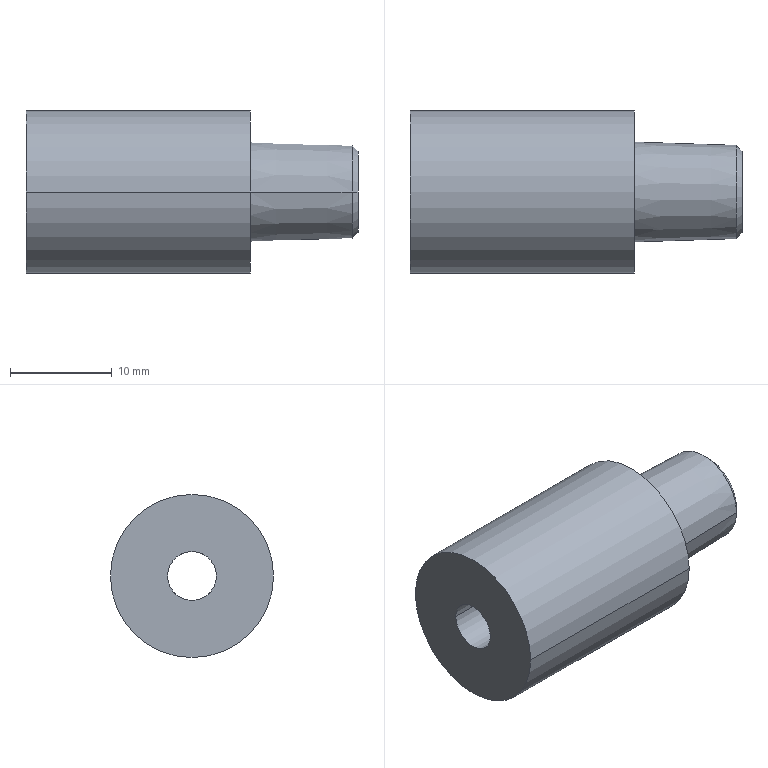Part | Creo | 1 solid | 21 faces | box 32.58 x 16 x 16 mm | volume 4565 mm3 | plane 11 | cylinder 6 | cone 4 | commonest cylinder face diameters 4.8 x4 16 x2
STEP:
#1=CARTESIAN_POINT('',(-305.,-184.66,90.));
#2=VERTEX_POINT('',#1);
#3=CARTESIAN_POINT('',(-305.,-175.5,90.));
#4=VERTEX_POINT('',#3);
#5=CARTESIAN_POINT('',(-305.,-180.08,90.));
#6=DIRECTION('',(-1.,0.,0.));
#7=DIRECTION('',(0.,-1.,0.));
#8=AXIS2_PLACEMENT_3D('',#5,#6,#7);
#9=CIRCLE('',#8,4.58);
#10=EDGE_CURVE('',#2,#4,#9,.T.);
#11=ORIENTED_EDGE('',*,*,#10,.F.);
#12=CARTESIAN_POINT('',(-315.,-184.98,90.));
#13=VERTEX_POINT('',#12);
#14=CARTESIAN_POINT('',(-305.,-184.66,90.));
#15=DIRECTION('',(-0.9995,-0.03198,0.));
#16=VECTOR('',#15,10.005);
#17=LINE('',#14,#16);
#18=EDGE_CURVE('',#2,#13,#17,.T.);
#19=ORIENTED_EDGE('',*,*,#18,.T.);
#20=CARTESIAN_POINT('',(-315.,-175.18,90.));
#21=VERTEX_POINT('',#20);
#22=CARTESIAN_POINT('',(-315.,-180.08,90.));
#23=DIRECTION('',(-1.,0.,0.));
#24=DIRECTION('',(0.,-1.,0.));
#25=AXIS2_PLACEMENT_3D('',#22,#23,#24);
#26=CIRCLE('',#25,4.9);
#27=EDGE_CURVE('',#13,#21,#26,.T.);
#28=ORIENTED_EDGE('',*,*,#27,.T.);
#29=CARTESIAN_POINT('',(-305.,-175.5,90.));
#30=DIRECTION('',(-0.9995,0.03198,0.));
#31=VECTOR('',#30,10.005);
#32=LINE('',#29,#31);
#33=EDGE_CURVE('',#4,#21,#32,.T.);
#34=ORIENTED_EDGE('',*,*,#33,.F.);
#35=EDGE_LOOP('',(#11,#19,#28,#34));
#36=FACE_OUTER_BOUND('',#35,.F.);
#37=CARTESIAN_POINT('',(-310.,-180.08,90.));
#38=DIRECTION('',(-1.,0.,0.));
#39=DIRECTION('',(0.,-1.,0.));
#40=AXIS2_PLACEMENT_3D('',#37,#38,#39);
#41=CONICAL_SURFACE('',#40,4.74,1.833);
#42=ADVANCED_FACE('',(#36),#41,.T.);
#43=CARTESIAN_POINT('',(-304.42,-176.08,90.));
#44=VERTEX_POINT('',#43);
#45=CARTESIAN_POINT('',(-304.42,-184.08,90.));
#46=VERTEX_POINT('',#45);
#47=CARTESIAN_POINT('',(-304.42,-180.08,90.));
#48=DIRECTION('',(1.,0.,0.));
#49=DIRECTION('',(0.,1.,0.));
#50=AXIS2_PLACEMENT_3D('',#47,#48,#49);
#51=CIRCLE('',#50,4.);
#52=EDGE_CURVE('',#44,#46,#51,.T.);
#53=ORIENTED_EDGE('',*,*,#52,.T.);
#54=CARTESIAN_POINT('',(-304.42,-184.08,90.));
#55=DIRECTION('',(-0.7071,-0.7071,0.));
#56=VECTOR('',#55,0.8202);
#57=LINE('',#54,#56);
#58=EDGE_CURVE('',#46,#2,#57,.T.);
#59=ORIENTED_EDGE('',*,*,#58,.T.);
#60=ORIENTED_EDGE('',*,*,#10,.T.);
#61=CARTESIAN_POINT('',(-304.42,-176.08,90.));
#62=DIRECTION('',(-0.7071,0.7071,0.));
#63=VECTOR('',#62,0.8202);
#64=LINE('',#61,#63);
#65=EDGE_CURVE('',#44,#4,#64,.T.);
#66=ORIENTED_EDGE('',*,*,#65,.F.);
#67=EDGE_LOOP('',(#53,#59,#60,#66));
#68=FACE_OUTER_BOUND('',#67,.F.);
#69=CARTESIAN_POINT('',(-304.71,-180.08,90.));
#70=DIRECTION('',(-1.,0.,0.));
#71=DIRECTION('',(0.,-1.,0.));
#72=AXIS2_PLACEMENT_3D('',#69,#70,#71);
#73=CONICAL_SURFACE('',#72,4.29,45.);
#74=ADVANCED_FACE('',(#68),#73,.T.);
#75=CARTESIAN_POINT('',(-304.42,-180.08,90.));
#76=DIRECTION('',(1.,0.,0.));
#77=DIRECTION('',(0.,-1.,0.));
#78=AXIS2_PLACEMENT_3D('',#75,#76,#77);
#79=CIRCLE('',#78,4.);
#80=EDGE_CURVE('',#46,#44,#79,.T.);
#81=ORIENTED_EDGE('',*,*,#80,.F.);
#82=ORIENTED_EDGE('',*,*,#52,.F.);
#83=EDGE_LOOP('',(#81,#82));
#84=FACE_OUTER_BOUND('',#83,.F.);
#85=CARTESIAN_POINT('',(-304.42,-180.08,87.6));
#86=VERTEX_POINT('',#85);
#87=CARTESIAN_POINT('',(-304.42,-182.48,90.));
#88=VERTEX_POINT('',#87);
#89=CARTESIAN_POINT('',(-304.42,-180.08,90.));
#90=DIRECTION('',(-1.,0.,0.));
#91=DIRECTION('',(0.,0.,-1.));
#92=AXIS2_PLACEMENT_3D('',#89,#90,#91);
#93=CIRCLE('',#92,2.4);
#94=EDGE_CURVE('',#86,#88,#93,.T.);
#95=ORIENTED_EDGE('',*,*,#94,.F.);
#96=CARTESIAN_POINT('',(-304.42,-177.68,90.));
#97=VERTEX_POINT('',#96);
#98=CARTESIAN_POINT('',(-304.42,-180.08,90.));
#99=DIRECTION('',(-1.,0.,0.));
#100=DIRECTION('',(0.,1.,0.));
#101=AXIS2_PLACEMENT_3D('',#98,#99,#100);
#102=CIRCLE('',#101,2.4);
#103=EDGE_CURVE('',#97,#86,#102,.T.);
#104=ORIENTED_EDGE('',*,*,#103,.F.);
#105=CARTESIAN_POINT('',(-304.42,-180.08,90.));
#106=DIRECTION('',(-1.,0.,0.));
#107=DIRECTION('',(0.,-1.,0.));
#108=AXIS2_PLACEMENT_3D('',#105,#106,#107);
#109=CIRCLE('',#108,2.4);
#110=EDGE_CURVE('',#88,#97,#109,.T.);
#111=ORIENTED_EDGE('',*,*,#110,.F.);
#112=EDGE_LOOP('',(#95,#104,#111));
#113=FACE_BOUND('',#112,.F.);
#114=CARTESIAN_POINT('',(-304.42,-180.08,90.));
#115=DIRECTION('',(1.,0.,0.));
#116=DIRECTION('',(0.,0.,-1.));
#117=AXIS2_PLACEMENT_3D('',#114,#115,#116);
#118=PLANE('',#117);
#119=ADVANCED_FACE('',(#84,#113),#118,.T.);
#120=ORIENTED_EDGE('',*,*,#103,.T.);
#121=ORIENTED_EDGE('',*,*,#94,.T.);
#122=CARTESIAN_POINT('',(-312.,-182.48,90.));
#123=VERTEX_POINT('',#122);
#124=CARTESIAN_POINT('',(-312.,-182.48,90.));
#125=DIRECTION('',(1.,0.,0.));
#126=VECTOR('',#125,7.58);
#127=LINE('',#124,#126);
#128=EDGE_CURVE('',#123,#88,#127,.T.);
#129=ORIENTED_EDGE('',*,*,#128,.F.);
#130=CARTESIAN_POINT('',(-312.,-180.08,87.6));
#131=VERTEX_POINT('',#130);
#132=CARTESIAN_POINT('',(-312.,-180.08,90.));
#133=DIRECTION('',(1.,0.,0.));
#134=DIRECTION('',(0.,-1.,0.));
#135=AXIS2_PLACEMENT_3D('',#132,#133,#134);
#136=CIRCLE('',#135,2.4);
#137=EDGE_CURVE('',#123,#131,#136,.T.);
#138=ORIENTED_EDGE('',*,*,#137,.T.);
#139=CARTESIAN_POINT('',(-312.,-177.68,90.));
#140=VERTEX_POINT('',#139);
#141=CARTESIAN_POINT('',(-312.,-180.08,90.));
#142=DIRECTION('',(1.,0.,0.));
#143=DIRECTION('',(0.,0.,-1.));
#144=AXIS2_PLACEMENT_3D('',#141,#142,#143);
#145=CIRCLE('',#144,2.4);
#146=EDGE_CURVE('',#131,#140,#145,.T.);
#147=ORIENTED_EDGE('',*,*,#146,.T.);
#148=CARTESIAN_POINT('',(-312.,-177.68,90.));
#149=DIRECTION('',(1.,0.,0.));
#150=VECTOR('',#149,7.58);
#151=LINE('',#148,#150);
#152=EDGE_CURVE('',#140,#97,#151,.T.);
#153=ORIENTED_EDGE('',*,*,#152,.T.);
#154=EDGE_LOOP('',(#120,#121,#129,#138,#147,#153));
#155=FACE_OUTER_BOUND('',#154,.F.);
#156=CARTESIAN_POINT('',(-124.,-180.08,90.));
#157=DIRECTION('',(1.,0.,0.));
#158=DIRECTION('',(0.,1.,0.));
#159=AXIS2_PLACEMENT_3D('',#156,#157,#158);
#160=CYLINDRICAL_SURFACE('',#159,2.4);
#161=ADVANCED_FACE('',(#155),#160,.F.);
#162=ORIENTED_EDGE('',*,*,#110,.T.);
#163=ORIENTED_EDGE('',*,*,#152,.F.);
#164=CARTESIAN_POINT('',(-312.,-180.08,92.4));
#165=VERTEX_POINT('',#164);
#166=CARTESIAN_POINT('',(-312.,-180.08,90.));
#167=DIRECTION('',(1.,0.,0.));
#168=DIRECTION('',(0.,1.,0.));
#169=AXIS2_PLACEMENT_3D('',#166,#167,#168);
#170=CIRCLE('',#169,2.4);
#171=EDGE_CURVE('',#140,#165,#170,.T.);
#172=ORIENTED_EDGE('',*,*,#171,.T.);
#173=CARTESIAN_POINT('',(-312.,-180.08,90.));
#174=DIRECTION('',(1.,0.,0.));
#175=DIRECTION('',(0.,0.,1.));
#176=AXIS2_PLACEMENT_3D('',#173,#174,#175);
#177=CIRCLE('',#176,2.4);
#178=EDGE_CURVE('',#165,#123,#177,.T.);
#179=ORIENTED_EDGE('',*,*,#178,.T.);
#180=ORIENTED_EDGE('',*,*,#128,.T.);
#181=EDGE_LOOP('',(#162,#163,#172,#179,#180));
#182=FACE_OUTER_BOUND('',#181,.F.);
#183=CARTESIAN_POINT('',(-124.,-180.08,90.));
#184=DIRECTION('',(1.,0.,0.));
#185=DIRECTION('',(0.,1.,0.));
#186=AXIS2_PLACEMENT_3D('',#183,#184,#185);
#187=CYLINDRICAL_SURFACE('',#186,2.4);
#188=ADVANCED_FACE('',(#182),#187,.F.);
#189=CARTESIAN_POINT('',(-312.,-182.53,91.415));
#190=VERTEX_POINT('',#189);
#191=CARTESIAN_POINT('',(-312.,-182.53,88.585));
#192=VERTEX_POINT('',#191);
#193=CARTESIAN_POINT('',(-312.,-182.53,91.415));
#194=DIRECTION('',(0.,0.,-1.));
#195=VECTOR('',#194,2.829);
#196=LINE('',#193,#195);
#197=EDGE_CURVE('',#190,#192,#196,.T.);
#198=ORIENTED_EDGE('',*,*,#197,.T.);
#199=CARTESIAN_POINT('',(-312.,-180.08,87.171));
#200=VERTEX_POINT('',#199);
#201=CARTESIAN_POINT('',(-312.,-180.08,87.171));
#202=DIRECTION('',(0.,-0.866,0.5));
#203=VECTOR('',#202,2.829);
#204=LINE('',#201,#203);
#205=EDGE_CURVE('',#200,#192,#204,.T.);
#206=ORIENTED_EDGE('',*,*,#205,.F.);
#207=CARTESIAN_POINT('',(-312.,-177.63,88.585));
#208=VERTEX_POINT('',#207);
#209=CARTESIAN_POINT('',(-312.,-177.63,88.585));
#210=DIRECTION('',(0.,-0.866,-0.5));
#211=VECTOR('',#210,2.829);
#212=LINE('',#209,#211);
#213=EDGE_CURVE('',#208,#200,#212,.T.);
#214=ORIENTED_EDGE('',*,*,#213,.F.);
#215=CARTESIAN_POINT('',(-312.,-177.63,91.415));
#216=VERTEX_POINT('',#215);
#217=CARTESIAN_POINT('',(-312.,-177.63,88.585));
#218=DIRECTION('',(0.,0.,1.));
#219=VECTOR('',#218,2.829);
#220=LINE('',#217,#219);
#221=EDGE_CURVE('',#208,#216,#220,.T.);
#222=ORIENTED_EDGE('',*,*,#221,.T.);
#223=CARTESIAN_POINT('',(-312.,-180.08,92.829));
#224=VERTEX_POINT('',#223);
#225=CARTESIAN_POINT('',(-312.,-180.08,92.829));
#226=DIRECTION('',(0.,0.866,-0.5));
#227=VECTOR('',#226,2.829);
#228=LINE('',#225,#227);
#229=EDGE_CURVE('',#224,#216,#228,.T.);
#230=ORIENTED_EDGE('',*,*,#229,.F.);
#231=CARTESIAN_POINT('',(-312.,-182.53,91.415));
#232=DIRECTION('',(0.,0.866,0.5));
#233=VECTOR('',#232,2.829);
#234=LINE('',#231,#233);
#235=EDGE_CURVE('',#190,#224,#234,.T.);
#236=ORIENTED_EDGE('',*,*,#235,.F.);
#237=EDGE_LOOP('',(#198,#206,#214,#222,#230,#236));
#238=FACE_OUTER_BOUND('',#237,.F.);
#239=ORIENTED_EDGE('',*,*,#146,.F.);
#240=ORIENTED_EDGE('',*,*,#137,.F.);
#241=ORIENTED_EDGE('',*,*,#178,.F.);
#242=ORIENTED_EDGE('',*,*,#171,.F.);
#243=EDGE_LOOP('',(#239,#240,#241,#242));
#244=FACE_BOUND('',#243,.F.);
#245=CARTESIAN_POINT('',(-312.,-180.08,90.));
#246=DIRECTION('',(1.,0.,0.));
#247=DIRECTION('',(0.,0.,-1.));
#248=AXIS2_PLACEMENT_3D('',#245,#246,#247);
#249=PLANE('',#248);
#250=ADVANCED_FACE('',(#238,#244),#249,.F.);
#251=ORIENTED_EDGE('',*,*,#197,.F.);
#252=CARTESIAN_POINT('',(-315.,-182.53,91.415));
#253=VERTEX_POINT('',#252);
#254=CARTESIAN_POINT('',(-315.,-182.53,91.415));
#255=DIRECTION('',(1.,0.,0.));
#256=VECTOR('',#255,3.);
#257=LINE('',#254,#256);
#258=EDGE_CURVE('',#253,#190,#257,.T.);
#259=ORIENTED_EDGE('',*,*,#258,.F.);
#260=CARTESIAN_POINT('',(-315.,-182.53,88.585));
#261=VERTEX_POINT('',#260);
#262=CARTESIAN_POINT('',(-315.,-182.53,88.585));
#263=DIRECTION('',(0.,0.,1.));
#264=VECTOR('',#263,2.829);
#265=LINE('',#262,#264);
#266=EDGE_CURVE('',#261,#253,#265,.T.);
#267=ORIENTED_EDGE('',*,*,#266,.F.);
#268=CARTESIAN_POINT('',(-315.,-182.53,88.585));
#269=DIRECTION('',(1.,0.,0.));
#270=VECTOR('',#269,3.);
#271=LINE('',#268,#270);
#272=EDGE_CURVE('',#261,#192,#271,.T.);
#273=ORIENTED_EDGE('',*,*,#272,.T.);
#274=EDGE_LOOP('',(#251,#259,#267,#273));
#275=FACE_OUTER_BOUND('',#274,.F.);
#276=CARTESIAN_POINT('',(-313.5,-182.53,90.));
#277=DIRECTION('',(0.,-1.,0.));
#278=DIRECTION('',(1.,0.,0.));
#279=AXIS2_PLACEMENT_3D('',#276,#277,#278);
#280=PLANE('',#279);
#281=ADVANCED_FACE('',(#275),#280,.F.);
#282=ORIENTED_EDGE('',*,*,#235,.T.);
#283=CARTESIAN_POINT('',(-315.,-180.08,92.829));
#284=VERTEX_POINT('',#283);
#285=CARTESIAN_POINT('',(-315.,-180.08,92.829));
#286=DIRECTION('',(1.,0.,0.));
#287=VECTOR('',#286,3.);
#288=LINE('',#285,#287);
#289=EDGE_CURVE('',#284,#224,#288,.T.);
#290=ORIENTED_EDGE('',*,*,#289,.F.);
#291=CARTESIAN_POINT('',(-315.,-180.08,92.829));
#292=DIRECTION('',(0.,-0.866,-0.5));
#293=VECTOR('',#292,2.829);
#294=LINE('',#291,#293);
#295=EDGE_CURVE('',#284,#253,#294,.T.);
#296=ORIENTED_EDGE('',*,*,#295,.T.);
#297=ORIENTED_EDGE('',*,*,#258,.T.);
#298=EDGE_LOOP('',(#282,#290,#296,#297));
#299=FACE_OUTER_BOUND('',#298,.F.);
#300=CARTESIAN_POINT('',(-313.5,-181.305,92.122));
#301=DIRECTION('',(0.,-0.5,0.866));
#302=DIRECTION('',(0.,-0.866,-0.5));
#303=AXIS2_PLACEMENT_3D('',#300,#301,#302);
#304=PLANE('',#303);
#305=ADVANCED_FACE('',(#299),#304,.F.);
#306=ORIENTED_EDGE('',*,*,#229,.T.);
#307=CARTESIAN_POINT('',(-315.,-177.63,91.415));
#308=VERTEX_POINT('',#307);
#309=CARTESIAN_POINT('',(-315.,-177.63,91.415));
#310=DIRECTION('',(1.,0.,0.));
#311=VECTOR('',#310,3.);
#312=LINE('',#309,#311);
#313=EDGE_CURVE('',#308,#216,#312,.T.);
#314=ORIENTED_EDGE('',*,*,#313,.F.);
#315=CARTESIAN_POINT('',(-315.,-177.63,91.415));
#316=DIRECTION('',(0.,-0.866,0.5));
#317=VECTOR('',#316,2.829);
#318=LINE('',#315,#317);
#319=EDGE_CURVE('',#308,#284,#318,.T.);
#320=ORIENTED_EDGE('',*,*,#319,.T.);
#321=ORIENTED_EDGE('',*,*,#289,.T.);
#322=EDGE_LOOP('',(#306,#314,#320,#321));
#323=FACE_OUTER_BOUND('',#322,.F.);
#324=CARTESIAN_POINT('',(-313.5,-178.855,92.122));
#325=DIRECTION('',(0.,0.5,0.866));
#326=DIRECTION('',(0.,-0.866,0.5));
#327=AXIS2_PLACEMENT_3D('',#324,#325,#326);
#328=PLANE('',#327);
#329=ADVANCED_FACE('',(#323),#328,.F.);
#330=ORIENTED_EDGE('',*,*,#221,.F.);
#331=CARTESIAN_POINT('',(-315.,-177.63,88.585));
#332=VERTEX_POINT('',#331);
#333=CARTESIAN_POINT('',(-315.,-177.63,88.585));
#334=DIRECTION('',(1.,0.,0.));
#335=VECTOR('',#334,3.);
#336=LINE('',#333,#335);
#337=EDGE_CURVE('',#332,#208,#336,.T.);
#338=ORIENTED_EDGE('',*,*,#337,.F.);
#339=CARTESIAN_POINT('',(-315.,-177.63,91.415));
#340=DIRECTION('',(0.,0.,-1.));
#341=VECTOR('',#340,2.829);
#342=LINE('',#339,#341);
#343=EDGE_CURVE('',#308,#332,#342,.T.);
#344=ORIENTED_EDGE('',*,*,#343,.F.);
#345=ORIENTED_EDGE('',*,*,#313,.T.);
#346=EDGE_LOOP('',(#330,#338,#344,#345));
#347=FACE_OUTER_BOUND('',#346,.F.);
#348=CARTESIAN_POINT('',(-313.5,-177.63,90.));
#349=DIRECTION('',(0.,1.,0.));
#350=DIRECTION('',(-1.,0.,0.));
#351=AXIS2_PLACEMENT_3D('',#348,#349,#350);
#352=PLANE('',#351);
#353=ADVANCED_FACE('',(#347),#352,.F.);
#354=ORIENTED_EDGE('',*,*,#213,.T.);
#355=CARTESIAN_POINT('',(-315.,-180.08,87.171));
#356=VERTEX_POINT('',#355);
#357=CARTESIAN_POINT('',(-315.,-180.08,87.171));
#358=DIRECTION('',(1.,0.,0.));
#359=VECTOR('',#358,3.);
#360=LINE('',#357,#359);
#361=EDGE_CURVE('',#356,#200,#360,.T.);
#362=ORIENTED_EDGE('',*,*,#361,.F.);
#363=CARTESIAN_POINT('',(-315.,-180.08,87.171));
#364=DIRECTION('',(0.,0.866,0.5));
#365=VECTOR('',#364,2.829);
#366=LINE('',#363,#365);
#367=EDGE_CURVE('',#356,#332,#366,.T.);
#368=ORIENTED_EDGE('',*,*,#367,.T.);
#369=ORIENTED_EDGE('',*,*,#337,.T.);
#370=EDGE_LOOP('',(#354,#362,#368,#369));
#371=FACE_OUTER_BOUND('',#370,.F.);
#372=CARTESIAN_POINT('',(-313.5,-178.855,87.878));
#373=DIRECTION('',(0.,0.5,-0.866));
#374=DIRECTION('',(0.,0.866,0.5));
#375=AXIS2_PLACEMENT_3D('',#372,#373,#374);
#376=PLANE('',#375);
#377=ADVANCED_FACE('',(#371),#376,.F.);
#378=ORIENTED_EDGE('',*,*,#205,.T.);
#379=ORIENTED_EDGE('',*,*,#272,.F.);
#380=CARTESIAN_POINT('',(-315.,-182.53,88.585));
#381=DIRECTION('',(0.,0.866,-0.5));
#382=VECTOR('',#381,2.829);
#383=LINE('',#380,#382);
#384=EDGE_CURVE('',#261,#356,#383,.T.);
#385=ORIENTED_EDGE('',*,*,#384,.T.);
#386=ORIENTED_EDGE('',*,*,#361,.T.);
#387=EDGE_LOOP('',(#378,#379,#385,#386));
#388=FACE_OUTER_BOUND('',#387,.F.);
#389=CARTESIAN_POINT('',(-313.5,-181.305,87.878));
#390=DIRECTION('',(0.,-0.5,-0.866));
#391=DIRECTION('',(0.,0.866,-0.5));
#392=AXIS2_PLACEMENT_3D('',#389,#390,#391);
#393=PLANE('',#392);
#394=ADVANCED_FACE('',(#388),#393,.F.);
#395=ORIENTED_EDGE('',*,*,#266,.T.);
#396=ORIENTED_EDGE('',*,*,#295,.F.);
#397=ORIENTED_EDGE('',*,*,#319,.F.);
#398=ORIENTED_EDGE('',*,*,#343,.T.);
#399=ORIENTED_EDGE('',*,*,#367,.F.);
#400=ORIENTED_EDGE('',*,*,#384,.F.);
#401=EDGE_LOOP('',(#395,#396,#397,#398,#399,#400));
#402=FACE_OUTER_BOUND('',#401,.F.);
#403=CARTESIAN_POINT('',(-315.,-180.08,87.6));
#404=VERTEX_POINT('',#403);
#405=CARTESIAN_POINT('',(-315.,-182.48,90.));
#406=VERTEX_POINT('',#405);
#407=CARTESIAN_POINT('',(-315.,-180.08,90.));
#408=DIRECTION('',(-1.,0.,0.));
#409=DIRECTION('',(0.,0.,-1.));
#410=AXIS2_PLACEMENT_3D('',#407,#408,#409);
#411=CIRCLE('',#410,2.4);
#412=EDGE_CURVE('',#404,#406,#411,.T.);
#413=ORIENTED_EDGE('',*,*,#412,.F.);
#414=CARTESIAN_POINT('',(-315.,-177.68,90.));
#415=VERTEX_POINT('',#414);
#416=CARTESIAN_POINT('',(-315.,-180.08,90.));
#417=DIRECTION('',(-1.,0.,0.));
#418=DIRECTION('',(0.,1.,0.));
#419=AXIS2_PLACEMENT_3D('',#416,#417,#418);
#420=CIRCLE('',#419,2.4);
#421=EDGE_CURVE('',#415,#404,#420,.T.);
#422=ORIENTED_EDGE('',*,*,#421,.F.);
#423=CARTESIAN_POINT('',(-315.,-180.08,90.));
#424=DIRECTION('',(-1.,0.,0.));
#425=DIRECTION('',(0.,-1.,0.));
#426=AXIS2_PLACEMENT_3D('',#423,#424,#425);
#427=CIRCLE('',#426,2.4);
#428=EDGE_CURVE('',#406,#415,#427,.T.);
#429=ORIENTED_EDGE('',*,*,#428,.F.);
#430=EDGE_LOOP('',(#413,#422,#429));
#431=FACE_BOUND('',#430,.F.);
#432=CARTESIAN_POINT('',(-315.,-180.08,90.));
#433=DIRECTION('',(1.,0.,0.));
#434=DIRECTION('',(0.,0.,-1.));
#435=AXIS2_PLACEMENT_3D('',#432,#433,#434);
#436=PLANE('',#435);
#437=ADVANCED_FACE('',(#402,#431),#436,.T.);
#438=ORIENTED_EDGE('',*,*,#421,.T.);
#439=ORIENTED_EDGE('',*,*,#412,.T.);
#440=CARTESIAN_POINT('',(-337.,-182.48,90.));
#441=VERTEX_POINT('',#440);
#442=CARTESIAN_POINT('',(-337.,-182.48,90.));
#443=DIRECTION('',(1.,0.,0.));
#444=VECTOR('',#443,22.);
#445=LINE('',#442,#444);
#446=EDGE_CURVE('',#441,#406,#445,.T.);
#447=ORIENTED_EDGE('',*,*,#446,.F.);
#448=CARTESIAN_POINT('',(-337.,-177.68,90.));
#449=VERTEX_POINT('',#448);
#450=CARTESIAN_POINT('',(-337.,-180.08,90.));
#451=DIRECTION('',(1.,0.,0.));
#452=DIRECTION('',(0.,-1.,0.));
#453=AXIS2_PLACEMENT_3D('',#450,#451,#452);
#454=CIRCLE('',#453,2.4);
#455=EDGE_CURVE('',#441,#449,#454,.T.);
#456=ORIENTED_EDGE('',*,*,#455,.T.);
#457=CARTESIAN_POINT('',(-337.,-177.68,90.));
#458=DIRECTION('',(1.,0.,0.));
#459=VECTOR('',#458,22.);
#460=LINE('',#457,#459);
#461=EDGE_CURVE('',#449,#415,#460,.T.);
#462=ORIENTED_EDGE('',*,*,#461,.T.);
#463=EDGE_LOOP('',(#438,#439,#447,#456,#462));
#464=FACE_OUTER_BOUND('',#463,.F.);
#465=CARTESIAN_POINT('',(-124.,-180.08,90.));
#466=DIRECTION('',(1.,0.,0.));
#467=DIRECTION('',(0.,1.,0.));
#468=AXIS2_PLACEMENT_3D('',#465,#466,#467);
#469=CYLINDRICAL_SURFACE('',#468,2.4);
#470=ADVANCED_FACE('',(#464),#469,.F.);
#471=ORIENTED_EDGE('',*,*,#428,.T.);
#472=ORIENTED_EDGE('',*,*,#461,.F.);
#473=CARTESIAN_POINT('',(-337.,-180.08,92.4));
#474=VERTEX_POINT('',#473);
#475=CARTESIAN_POINT('',(-337.,-180.08,90.));
#476=DIRECTION('',(1.,0.,0.));
#477=DIRECTION('',(0.,1.,0.));
#478=AXIS2_PLACEMENT_3D('',#475,#476,#477);
#479=CIRCLE('',#478,2.4);
#480=EDGE_CURVE('',#449,#474,#479,.T.);
#481=ORIENTED_EDGE('',*,*,#480,.T.);
#482=CARTESIAN_POINT('',(-337.,-180.08,90.));
#483=DIRECTION('',(1.,0.,0.));
#484=DIRECTION('',(0.,0.,1.));
#485=AXIS2_PLACEMENT_3D('',#482,#483,#484);
#486=CIRCLE('',#485,2.4);
#487=EDGE_CURVE('',#474,#441,#486,.T.);
#488=ORIENTED_EDGE('',*,*,#487,.T.);
#489=ORIENTED_EDGE('',*,*,#446,.T.);
#490=EDGE_LOOP('',(#471,#472,#481,#488,#489));
#491=FACE_OUTER_BOUND('',#490,.F.);
#492=CARTESIAN_POINT('',(-124.,-180.08,90.));
#493=DIRECTION('',(1.,0.,0.));
#494=DIRECTION('',(0.,1.,0.));
#495=AXIS2_PLACEMENT_3D('',#492,#493,#494);
#496=CYLINDRICAL_SURFACE('',#495,2.4);
#497=ADVANCED_FACE('',(#491),#496,.F.);
#498=CARTESIAN_POINT('',(-337.,-180.08,98.));
#499=VERTEX_POINT('',#498);
#500=CARTESIAN_POINT('',(-337.,-172.08,90.));
#501=VERTEX_POINT('',#500);
#502=CARTESIAN_POINT('',(-337.,-180.08,90.));
#503=DIRECTION('',(-1.,0.,0.));
#504=DIRECTION('',(0.,0.,1.));
#505=AXIS2_PLACEMENT_3D('',#502,#503,#504);
#506=CIRCLE('',#505,8.);
#507=EDGE_CURVE('',#499,#501,#506,.T.);
#508=ORIENTED_EDGE('',*,*,#507,.F.);
#509=CARTESIAN_POINT('',(-337.,-188.08,90.));
#510=VERTEX_POINT('',#509);
#511=CARTESIAN_POINT('',(-337.,-180.08,90.));
#512=DIRECTION('',(-1.,0.,0.));
#513=DIRECTION('',(0.,-1.,0.));
#514=AXIS2_PLACEMENT_3D('',#511,#512,#513);
#515=CIRCLE('',#514,8.);
#516=EDGE_CURVE('',#510,#499,#515,.T.);
#517=ORIENTED_EDGE('',*,*,#516,.F.);
#518=CARTESIAN_POINT('',(-337.,-180.08,90.));
#519=DIRECTION('',(-1.,0.,0.));
#520=DIRECTION('',(0.,1.,0.));
#521=AXIS2_PLACEMENT_3D('',#518,#519,#520);
#522=CIRCLE('',#521,8.);
#523=EDGE_CURVE('',#501,#510,#522,.T.);
#524=ORIENTED_EDGE('',*,*,#523,.F.);
#525=EDGE_LOOP('',(#508,#517,#524));
#526=FACE_OUTER_BOUND('',#525,.F.);
#527=ORIENTED_EDGE('',*,*,#487,.F.);
#528=ORIENTED_EDGE('',*,*,#480,.F.);
#529=ORIENTED_EDGE('',*,*,#455,.F.);
#530=EDGE_LOOP('',(#527,#528,#529));
#531=FACE_BOUND('',#530,.F.);
#532=CARTESIAN_POINT('',(-337.,-180.08,90.));
#533=DIRECTION('',(-1.,0.,0.));
#534=DIRECTION('',(0.,0.,1.));
#535=AXIS2_PLACEMENT_3D('',#532,#533,#534);
#536=PLANE('',#535);
#537=ADVANCED_FACE('',(#526,#531),#536,.T.);
#538=ORIENTED_EDGE('',*,*,#516,.T.);
#539=ORIENTED_EDGE('',*,*,#507,.T.);
#540=CARTESIAN_POINT('',(-315.,-172.08,90.));
#541=VERTEX_POINT('',#540);
#542=CARTESIAN_POINT('',(-315.,-172.08,90.));
#543=DIRECTION('',(-1.,0.,0.));
#544=VECTOR('',#543,22.);
#545=LINE('',#542,#544);
#546=EDGE_CURVE('',#541,#501,#545,.T.);
#547=ORIENTED_EDGE('',*,*,#546,.F.);
#548=CARTESIAN_POINT('',(-315.,-188.08,90.));
#549=VERTEX_POINT('',#548);
#550=CARTESIAN_POINT('',(-315.,-180.08,90.));
#551=DIRECTION('',(1.,0.,0.));
#552=DIRECTION('',(0.,1.,0.));
#553=AXIS2_PLACEMENT_3D('',#550,#551,#552);
#554=CIRCLE('',#553,8.);
#555=EDGE_CURVE('',#541,#549,#554,.T.);
#556=ORIENTED_EDGE('',*,*,#555,.T.);
#557=CARTESIAN_POINT('',(-315.,-188.08,90.));
#558=DIRECTION('',(-1.,0.,0.));
#559=VECTOR('',#558,22.);
#560=LINE('',#557,#559);
#561=EDGE_CURVE('',#549,#510,#560,.T.);
#562=ORIENTED_EDGE('',*,*,#561,.T.);
#563=EDGE_LOOP('',(#538,#539,#547,#556,#562));
#564=FACE_OUTER_BOUND('',#563,.F.);
#565=CARTESIAN_POINT('',(-315.,-180.08,90.));
#566=DIRECTION('',(-1.,0.,0.));
#567=DIRECTION('',(0.,-1.,0.));
#568=AXIS2_PLACEMENT_3D('',#565,#566,#567);
#569=CYLINDRICAL_SURFACE('',#568,8.);
#570=ADVANCED_FACE('',(#564),#569,.T.);
#571=ORIENTED_EDGE('',*,*,#523,.T.);
#572=ORIENTED_EDGE('',*,*,#561,.F.);
#573=CARTESIAN_POINT('',(-315.,-180.08,82.));
#574=VERTEX_POINT('',#573);
#575=CARTESIAN_POINT('',(-315.,-180.08,90.));
#576=DIRECTION('',(1.,0.,0.));
#577=DIRECTION('',(0.,-1.,0.));
#578=AXIS2_PLACEMENT_3D('',#575,#576,#577);
#579=CIRCLE('',#578,8.);
#580=EDGE_CURVE('',#549,#574,#579,.T.);
#581=ORIENTED_EDGE('',*,*,#580,.T.);
#582=CARTESIAN_POINT('',(-315.,-180.08,90.));
#583=DIRECTION('',(1.,0.,0.));
#584=DIRECTION('',(0.,0.,-1.));
#585=AXIS2_PLACEMENT_3D('',#582,#583,#584);
#586=CIRCLE('',#585,8.);
#587=EDGE_CURVE('',#574,#541,#586,.T.);
#588=ORIENTED_EDGE('',*,*,#587,.T.);
#589=ORIENTED_EDGE('',*,*,#546,.T.);
#590=EDGE_LOOP('',(#571,#572,#581,#588,#589));
#591=FACE_OUTER_BOUND('',#590,.F.);
#592=CARTESIAN_POINT('',(-315.,-180.08,90.));
#593=DIRECTION('',(-1.,0.,0.));
#594=DIRECTION('',(0.,-1.,0.));
#595=AXIS2_PLACEMENT_3D('',#592,#593,#594);
#596=CYLINDRICAL_SURFACE('',#595,8.);
#597=ADVANCED_FACE('',(#591),#596,.T.);
#598=ORIENTED_EDGE('',*,*,#587,.F.);
#599=ORIENTED_EDGE('',*,*,#580,.F.);
#600=ORIENTED_EDGE('',*,*,#555,.F.);
#601=EDGE_LOOP('',(#598,#599,#600));
#602=FACE_OUTER_BOUND('',#601,.F.);
#603=ORIENTED_EDGE('',*,*,#27,.F.);
#604=CARTESIAN_POINT('',(-315.,-180.08,90.));
#605=DIRECTION('',(-1.,0.,0.));
#606=DIRECTION('',(0.,1.,0.));
#607=AXIS2_PLACEMENT_3D('',#604,#605,#606);
#608=CIRCLE('',#607,4.9);
#609=EDGE_CURVE('',#21,#13,#608,.T.);
#610=ORIENTED_EDGE('',*,*,#609,.F.);
#611=EDGE_LOOP('',(#603,#610));
#612=FACE_BOUND('',#611,.F.);
#613=CARTESIAN_POINT('',(-315.,-180.08,90.));
#614=DIRECTION('',(1.,0.,0.));
#615=DIRECTION('',(0.,0.,-1.));
#616=AXIS2_PLACEMENT_3D('',#613,#614,#615);
#617=PLANE('',#616);
#618=ADVANCED_FACE('',(#602,#612),#617,.T.);
#619=CARTESIAN_POINT('',(-305.,-180.08,90.));
#620=DIRECTION('',(-1.,0.,0.));
#621=DIRECTION('',(0.,1.,0.));
#622=AXIS2_PLACEMENT_3D('',#619,#620,#621);
#623=CIRCLE('',#622,4.58);
#624=EDGE_CURVE('',#4,#2,#623,.T.);
#625=ORIENTED_EDGE('',*,*,#624,.F.);
#626=ORIENTED_EDGE('',*,*,#33,.T.);
#627=ORIENTED_EDGE('',*,*,#609,.T.);
#628=ORIENTED_EDGE('',*,*,#18,.F.);
#629=EDGE_LOOP('',(#625,#626,#627,#628));
#630=FACE_OUTER_BOUND('',#629,.F.);
#631=CARTESIAN_POINT('',(-310.,-180.08,90.));
#632=DIRECTION('',(-1.,0.,0.));
#633=DIRECTION('',(0.,-1.,0.));
#634=AXIS2_PLACEMENT_3D('',#631,#632,#633);
#635=CONICAL_SURFACE('',#634,4.74,1.833);
#636=ADVANCED_FACE('',(#630),#635,.T.);
#637=ORIENTED_EDGE('',*,*,#80,.T.);
#638=ORIENTED_EDGE('',*,*,#65,.T.);
#639=ORIENTED_EDGE('',*,*,#624,.T.);
#640=ORIENTED_EDGE('',*,*,#58,.F.);
#641=EDGE_LOOP('',(#637,#638,#639,#640));
#642=FACE_OUTER_BOUND('',#641,.F.);
#643=CARTESIAN_POINT('',(-304.71,-180.08,90.));
#644=DIRECTION('',(-1.,0.,0.));
#645=DIRECTION('',(0.,-1.,0.));
#646=AXIS2_PLACEMENT_3D('',#643,#644,#645);
#647=CONICAL_SURFACE('',#646,4.29,45.);
#648=ADVANCED_FACE('',(#642),#647,.T.);
#649=CLOSED_SHELL('',(#42,#74,#119,#161,#188,#250,#281,#305,#329,#353,#377,#394,#437,#470,#497,#537,#570,#597,#618,#636,#648));
#650=MANIFOLD_SOLID_BREP('',#649);
#651=(LENGTH_UNIT()NAMED_UNIT(*)SI_UNIT(.MILLI.,.METRE.));
#652=UNCERTAINTY_MEASURE_WITH_UNIT(LENGTH_MEASURE(0.003967),#651,'','');
#653=(NAMED_UNIT(*)PLANE_ANGLE_UNIT()SI_UNIT($,.RADIAN.));
#654=PLANE_ANGLE_MEASURE_WITH_UNIT(PLANE_ANGLE_MEASURE(0.01745),#653);
#655=(CONVERSION_BASED_UNIT('DEGREE',#654)NAMED_UNIT(*)PLANE_ANGLE_UNIT());
#656=(NAMED_UNIT(*)SI_UNIT($,.STERADIAN.)SOLID_ANGLE_UNIT());
#657=(GEOMETRIC_REPRESENTATION_CONTEXT(3)GLOBAL_UNCERTAINTY_ASSIGNED_CONTEXT((#652))GLOBAL_UNIT_ASSIGNED_CONTEXT((#651,#655,#656))REPRESENTATION_CONTEXT('',''));
#658=ADVANCED_BREP_SHAPE_REPRESENTATION('',(#650),#657);